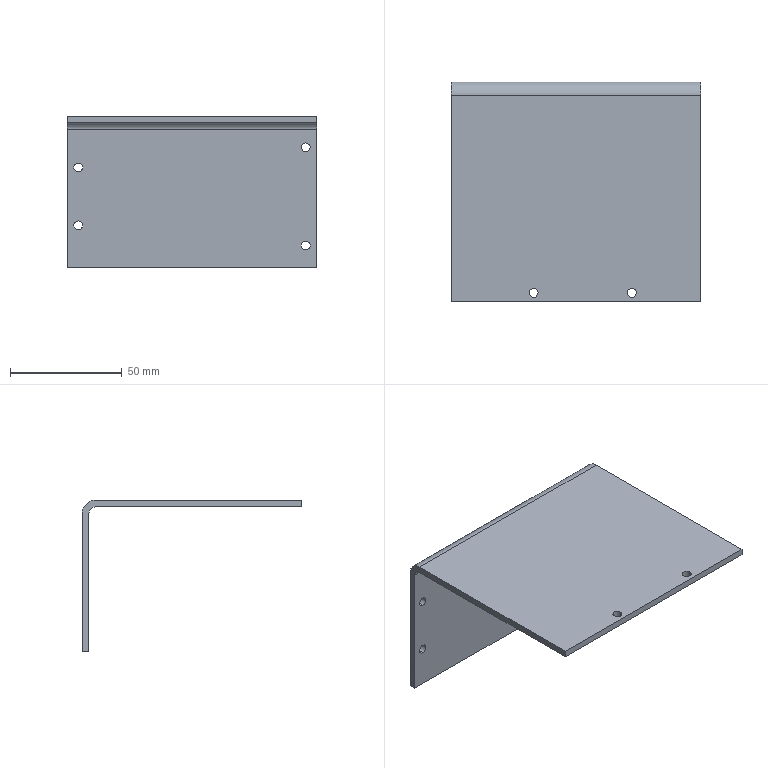Part | STEP file | 0243_225_Cover | 1 solid | 22 faces | box 112 x 98.5 x 68 mm | volume 54061 mm3 | cylinder 14 | plane 8 | commonest cylinder face diameters 4 x12 6 x1 12 x1